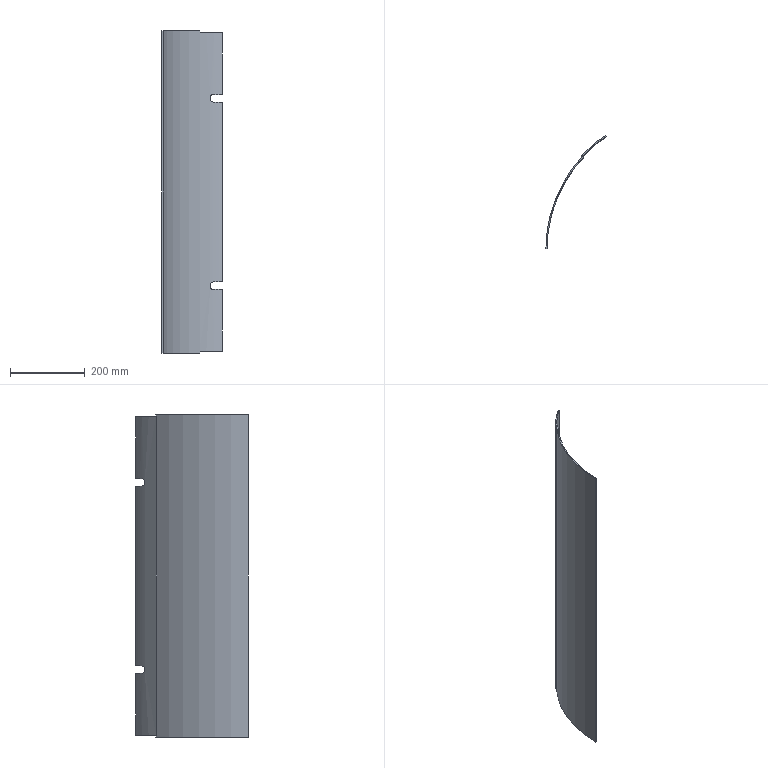Part | NX | features BREP 1 | 1 solid | 20 faces | box 160.623 x 300.85 x 860 mm | volume 907934 mm3 | plane 14 | cylinder 6 | commonest cylinder face diameters 20 x2 726 x2 720 x1 732 x1
STEP:
#1=CARTESIAN_POINT('',(-226.352,283.784,-260.));
#2=VERTEX_POINT('',#1);
#3=CARTESIAN_POINT('',(-226.352,283.784,-240.));
#4=VERTEX_POINT('',#3);
#5=CARTESIAN_POINT('',(-226.352,283.784,-260.));
#6=CARTESIAN_POINT('',(-228.418,282.137,-260.));
#7=CARTESIAN_POINT('',(-232.425,278.852,-257.834));
#8=CARTESIAN_POINT('',(-234.913,276.736,-250.009));
#9=CARTESIAN_POINT('',(-232.432,278.847,-242.169));
#10=CARTESIAN_POINT('',(-228.418,282.137,-240.));
#11=CARTESIAN_POINT('',(-226.352,283.784,-240.));
#12=B_SPLINE_CURVE_WITH_KNOTS('',3,(#5,#6,#7,#8,#9,#10,#11),.UNSPECIFIED.,.F.,.F.,(4,1,1,1,4),(0.,0.007816,0.01563,0.02345,0.03126),.UNSPECIFIED.);
#13=EDGE_CURVE('',#2,#4,#12,.T.);
#14=ORIENTED_EDGE('',*,*,#13,.T.);
#15=CARTESIAN_POINT('',(-202.365,301.36,-240.));
#16=VERTEX_POINT('',#15);
#17=CARTESIAN_POINT('',(0.,0.,-240.));
#18=DIRECTION('',(0.,0.,-1.));
#19=DIRECTION('',(-1.,0.,0.));
#20=AXIS2_PLACEMENT_3D('',#17,#18,#19);
#21=CIRCLE('',#20,363.);
#22=EDGE_CURVE('',#4,#16,#21,.T.);
#23=ORIENTED_EDGE('',*,*,#22,.T.);
#24=CARTESIAN_POINT('',(-202.365,301.36,240.));
#25=VERTEX_POINT('',#24);
#26=CARTESIAN_POINT('',(-202.365,301.36,430.));
#27=DIRECTION('',(0.,0.,-1.));
#28=VECTOR('',#27,1000.);
#29=LINE('',#26,#28);
#30=EDGE_CURVE('',#25,#16,#29,.T.);
#31=ORIENTED_EDGE('',*,*,#30,.F.);
#32=CARTESIAN_POINT('',(-226.352,283.784,240.));
#33=VERTEX_POINT('',#32);
#34=CARTESIAN_POINT('',(0.,0.,240.));
#35=DIRECTION('',(0.,0.,1.));
#36=DIRECTION('',(1.,0.,0.));
#37=AXIS2_PLACEMENT_3D('',#34,#35,#36);
#38=CIRCLE('',#37,363.);
#39=EDGE_CURVE('',#25,#33,#38,.T.);
#40=ORIENTED_EDGE('',*,*,#39,.T.);
#41=CARTESIAN_POINT('',(-226.352,283.784,260.));
#42=VERTEX_POINT('',#41);
#43=CARTESIAN_POINT('',(-226.352,283.784,240.));
#44=CARTESIAN_POINT('',(-228.418,282.137,240.));
#45=CARTESIAN_POINT('',(-232.425,278.852,242.166));
#46=CARTESIAN_POINT('',(-234.913,276.736,249.991));
#47=CARTESIAN_POINT('',(-232.432,278.847,257.831));
#48=CARTESIAN_POINT('',(-228.418,282.137,260.));
#49=CARTESIAN_POINT('',(-226.352,283.784,260.));
#50=B_SPLINE_CURVE_WITH_KNOTS('',3,(#43,#44,#45,#46,#47,#48,#49),.UNSPECIFIED.,.F.,.F.,(4,1,1,1,4),(0.,0.007816,0.01563,0.02345,0.03126),.UNSPECIFIED.);
#51=EDGE_CURVE('',#33,#42,#50,.T.);
#52=ORIENTED_EDGE('',*,*,#51,.T.);
#53=CARTESIAN_POINT('',(-202.365,301.36,260.));
#54=VERTEX_POINT('',#53);
#55=CARTESIAN_POINT('',(0.,0.,260.));
#56=DIRECTION('',(0.,0.,-1.));
#57=DIRECTION('',(-1.,0.,0.));
#58=AXIS2_PLACEMENT_3D('',#55,#56,#57);
#59=CIRCLE('',#58,363.);
#60=EDGE_CURVE('',#42,#54,#59,.T.);
#61=ORIENTED_EDGE('',*,*,#60,.T.);
#62=CARTESIAN_POINT('',(-202.365,301.36,425.));
#63=VERTEX_POINT('',#62);
#64=CARTESIAN_POINT('',(-202.365,301.36,430.));
#65=DIRECTION('',(0.,0.,-1.));
#66=VECTOR('',#65,1000.);
#67=LINE('',#64,#66);
#68=EDGE_CURVE('',#63,#54,#67,.T.);
#69=ORIENTED_EDGE('',*,*,#68,.F.);
#70=CARTESIAN_POINT('',(-263.653,249.511,425.));
#71=VERTEX_POINT('',#70);
#72=CARTESIAN_POINT('',(0.,0.,425.));
#73=DIRECTION('',(0.,0.,-1.));
#74=DIRECTION('',(1.,0.,0.));
#75=AXIS2_PLACEMENT_3D('',#72,#73,#74);
#76=CIRCLE('',#75,363.);
#77=EDGE_CURVE('',#71,#63,#76,.T.);
#78=ORIENTED_EDGE('',*,*,#77,.F.);
#79=CARTESIAN_POINT('',(-263.653,249.511,-425.));
#80=VERTEX_POINT('',#79);
#81=CARTESIAN_POINT('',(-263.653,249.511,430.));
#82=DIRECTION('',(0.,0.,-1.));
#83=VECTOR('',#82,1000.);
#84=LINE('',#81,#83);
#85=EDGE_CURVE('',#71,#80,#84,.T.);
#86=ORIENTED_EDGE('',*,*,#85,.T.);
#87=CARTESIAN_POINT('',(-202.365,301.36,-425.));
#88=VERTEX_POINT('',#87);
#89=CARTESIAN_POINT('',(0.,0.,-425.));
#90=DIRECTION('',(0.,0.,-1.));
#91=DIRECTION('',(1.,0.,0.));
#92=AXIS2_PLACEMENT_3D('',#89,#90,#91);
#93=CIRCLE('',#92,363.);
#94=EDGE_CURVE('',#80,#88,#93,.T.);
#95=ORIENTED_EDGE('',*,*,#94,.T.);
#96=CARTESIAN_POINT('',(-202.365,301.36,-260.));
#97=VERTEX_POINT('',#96);
#98=CARTESIAN_POINT('',(-202.365,301.36,430.));
#99=DIRECTION('',(0.,0.,-1.));
#100=VECTOR('',#99,1000.);
#101=LINE('',#98,#100);
#102=EDGE_CURVE('',#97,#88,#101,.T.);
#103=ORIENTED_EDGE('',*,*,#102,.F.);
#104=CARTESIAN_POINT('',(0.,0.,-260.));
#105=DIRECTION('',(0.,0.,1.));
#106=DIRECTION('',(1.,0.,0.));
#107=AXIS2_PLACEMENT_3D('',#104,#105,#106);
#108=CIRCLE('',#107,363.);
#109=EDGE_CURVE('',#97,#2,#108,.T.);
#110=ORIENTED_EDGE('',*,*,#109,.T.);
#111=EDGE_LOOP('',(#14,#23,#31,#40,#52,#61,#69,#78,#86,#95,#103,#110));
#112=FACE_BOUND('',#111,.T.);
#113=CARTESIAN_POINT('',(0.,0.,430.));
#114=DIRECTION('',(0.,0.,-1.));
#115=DIRECTION('',(1.,0.,0.));
#116=AXIS2_PLACEMENT_3D('',#113,#114,#115);
#117=CYLINDRICAL_SURFACE('',#116,363.);
#118=ADVANCED_FACE('',(#112),#117,.F.);
#119=ORIENTED_EDGE('',*,*,#30,.T.);
#120=CARTESIAN_POINT('',(-204.037,303.85,-240.));
#121=VERTEX_POINT('',#120);
#122=CARTESIAN_POINT('',(-204.037,303.85,-240.));
#123=DIRECTION('',(-0.5575,0.8302,0.));
#124=VECTOR('',#123,1000.);
#125=LINE('',#122,#124);
#126=EDGE_CURVE('',#16,#121,#125,.T.);
#127=ORIENTED_EDGE('',*,*,#126,.T.);
#128=CARTESIAN_POINT('',(-204.037,303.85,240.));
#129=VERTEX_POINT('',#128);
#130=CARTESIAN_POINT('',(-204.037,303.85,430.));
#131=DIRECTION('',(0.,0.,-1.));
#132=VECTOR('',#131,1000.);
#133=LINE('',#130,#132);
#134=EDGE_CURVE('',#129,#121,#133,.T.);
#135=ORIENTED_EDGE('',*,*,#134,.F.);
#136=CARTESIAN_POINT('',(-204.037,303.85,240.));
#137=DIRECTION('',(0.5575,-0.8302,0.));
#138=VECTOR('',#137,1000.);
#139=LINE('',#136,#138);
#140=EDGE_CURVE('',#129,#25,#139,.T.);
#141=ORIENTED_EDGE('',*,*,#140,.T.);
#142=EDGE_LOOP('',(#119,#127,#135,#141));
#143=FACE_BOUND('',#142,.T.);
#144=CARTESIAN_POINT('',(-204.037,303.85,430.));
#145=DIRECTION('',(0.8302,0.5575,0.));
#146=DIRECTION('',(0.5575,-0.8302,0.));
#147=AXIS2_PLACEMENT_3D('',#144,#145,#146);
#148=PLANE('',#147);
#149=ADVANCED_FACE('',(#143),#148,.T.);
#150=CARTESIAN_POINT('',(-204.037,303.85,-260.));
#151=VERTEX_POINT('',#150);
#152=CARTESIAN_POINT('',(-204.037,303.85,-425.));
#153=VERTEX_POINT('',#152);
#154=CARTESIAN_POINT('',(-204.037,303.85,430.));
#155=DIRECTION('',(0.,0.,-1.));
#156=VECTOR('',#155,1000.);
#157=LINE('',#154,#156);
#158=EDGE_CURVE('',#151,#153,#157,.T.);
#159=ORIENTED_EDGE('',*,*,#158,.F.);
#160=CARTESIAN_POINT('',(-204.037,303.85,-260.));
#161=DIRECTION('',(0.5575,-0.8302,0.));
#162=VECTOR('',#161,1000.);
#163=LINE('',#160,#162);
#164=EDGE_CURVE('',#151,#97,#163,.T.);
#165=ORIENTED_EDGE('',*,*,#164,.T.);
#166=ORIENTED_EDGE('',*,*,#102,.T.);
#167=CARTESIAN_POINT('',(-204.037,303.85,-425.));
#168=DIRECTION('',(-0.5575,0.8302,0.));
#169=VECTOR('',#168,1000.);
#170=LINE('',#167,#169);
#171=EDGE_CURVE('',#88,#153,#170,.T.);
#172=ORIENTED_EDGE('',*,*,#171,.T.);
#173=EDGE_LOOP('',(#159,#165,#166,#172));
#174=FACE_BOUND('',#173,.T.);
#175=CARTESIAN_POINT('',(-204.037,303.85,430.));
#176=DIRECTION('',(0.8302,0.5575,0.));
#177=DIRECTION('',(0.5575,-0.8302,0.));
#178=AXIS2_PLACEMENT_3D('',#175,#176,#177);
#179=PLANE('',#178);
#180=ADVANCED_FACE('',(#174),#179,.T.);
#181=CARTESIAN_POINT('',(-228.301,286.068,-240.));
#182=VERTEX_POINT('',#181);
#183=CARTESIAN_POINT('',(0.,0.,-240.));
#184=DIRECTION('',(0.,0.,-1.));
#185=DIRECTION('',(-1.,0.,0.));
#186=AXIS2_PLACEMENT_3D('',#183,#184,#185);
#187=CIRCLE('',#186,366.);
#188=EDGE_CURVE('',#182,#121,#187,.T.);
#189=ORIENTED_EDGE('',*,*,#188,.F.);
#190=CARTESIAN_POINT('',(-228.301,286.068,-260.));
#191=VERTEX_POINT('',#190);
#192=CARTESIAN_POINT('',(-228.301,286.068,-260.));
#193=CARTESIAN_POINT('',(-230.366,284.42,-260.));
#194=CARTESIAN_POINT('',(-234.373,281.135,-257.834));
#195=CARTESIAN_POINT('',(-236.86,279.018,-250.009));
#196=CARTESIAN_POINT('',(-234.379,281.129,-242.169));
#197=CARTESIAN_POINT('',(-230.366,284.42,-240.));
#198=CARTESIAN_POINT('',(-228.301,286.068,-240.));
#199=B_SPLINE_CURVE_WITH_KNOTS('',3,(#192,#193,#194,#195,#196,#197,#198),.UNSPECIFIED.,.F.,.F.,(4,1,1,1,4),(0.,0.007816,0.01563,0.02345,0.03126),.UNSPECIFIED.);
#200=EDGE_CURVE('',#191,#182,#199,.T.);
#201=ORIENTED_EDGE('',*,*,#200,.F.);
#202=CARTESIAN_POINT('',(0.,0.,-260.));
#203=DIRECTION('',(0.,0.,1.));
#204=DIRECTION('',(1.,0.,0.));
#205=AXIS2_PLACEMENT_3D('',#202,#203,#204);
#206=CIRCLE('',#205,366.);
#207=EDGE_CURVE('',#151,#191,#206,.T.);
#208=ORIENTED_EDGE('',*,*,#207,.F.);
#209=ORIENTED_EDGE('',*,*,#158,.T.);
#210=CARTESIAN_POINT('',(-267.83,249.445,-425.));
#211=VERTEX_POINT('',#210);
#212=CARTESIAN_POINT('',(0.,0.,-425.));
#213=DIRECTION('',(0.,0.,1.));
#214=DIRECTION('',(1.,0.,0.));
#215=AXIS2_PLACEMENT_3D('',#212,#213,#214);
#216=CIRCLE('',#215,366.);
#217=EDGE_CURVE('',#153,#211,#216,.T.);
#218=ORIENTED_EDGE('',*,*,#217,.T.);
#219=CARTESIAN_POINT('',(-267.83,249.445,425.));
#220=VERTEX_POINT('',#219);
#221=CARTESIAN_POINT('',(-267.83,249.445,430.));
#222=DIRECTION('',(0.,0.,-1.));
#223=VECTOR('',#222,1000.);
#224=LINE('',#221,#223);
#225=EDGE_CURVE('',#220,#211,#224,.T.);
#226=ORIENTED_EDGE('',*,*,#225,.F.);
#227=CARTESIAN_POINT('',(-204.037,303.85,425.));
#228=VERTEX_POINT('',#227);
#229=CARTESIAN_POINT('',(0.,0.,425.));
#230=DIRECTION('',(0.,0.,1.));
#231=DIRECTION('',(1.,0.,0.));
#232=AXIS2_PLACEMENT_3D('',#229,#230,#231);
#233=CIRCLE('',#232,366.);
#234=EDGE_CURVE('',#228,#220,#233,.T.);
#235=ORIENTED_EDGE('',*,*,#234,.F.);
#236=CARTESIAN_POINT('',(-204.037,303.85,260.));
#237=VERTEX_POINT('',#236);
#238=CARTESIAN_POINT('',(-204.037,303.85,430.));
#239=DIRECTION('',(0.,0.,-1.));
#240=VECTOR('',#239,1000.);
#241=LINE('',#238,#240);
#242=EDGE_CURVE('',#228,#237,#241,.T.);
#243=ORIENTED_EDGE('',*,*,#242,.T.);
#244=CARTESIAN_POINT('',(-228.301,286.068,260.));
#245=VERTEX_POINT('',#244);
#246=CARTESIAN_POINT('',(0.,0.,260.));
#247=DIRECTION('',(0.,0.,-1.));
#248=DIRECTION('',(-1.,0.,0.));
#249=AXIS2_PLACEMENT_3D('',#246,#247,#248);
#250=CIRCLE('',#249,366.);
#251=EDGE_CURVE('',#245,#237,#250,.T.);
#252=ORIENTED_EDGE('',*,*,#251,.F.);
#253=CARTESIAN_POINT('',(-228.301,286.068,240.));
#254=VERTEX_POINT('',#253);
#255=CARTESIAN_POINT('',(-228.301,286.068,240.));
#256=CARTESIAN_POINT('',(-230.366,284.42,240.));
#257=CARTESIAN_POINT('',(-234.373,281.135,242.166));
#258=CARTESIAN_POINT('',(-236.86,279.018,249.991));
#259=CARTESIAN_POINT('',(-234.379,281.129,257.831));
#260=CARTESIAN_POINT('',(-230.366,284.42,260.));
#261=CARTESIAN_POINT('',(-228.301,286.068,260.));
#262=B_SPLINE_CURVE_WITH_KNOTS('',3,(#255,#256,#257,#258,#259,#260,#261),.UNSPECIFIED.,.F.,.F.,(4,1,1,1,4),(0.,0.007816,0.01563,0.02345,0.03126),.UNSPECIFIED.);
#263=EDGE_CURVE('',#254,#245,#262,.T.);
#264=ORIENTED_EDGE('',*,*,#263,.F.);
#265=CARTESIAN_POINT('',(0.,0.,240.));
#266=DIRECTION('',(0.,0.,1.));
#267=DIRECTION('',(1.,0.,0.));
#268=AXIS2_PLACEMENT_3D('',#265,#266,#267);
#269=CIRCLE('',#268,366.);
#270=EDGE_CURVE('',#129,#254,#269,.T.);
#271=ORIENTED_EDGE('',*,*,#270,.F.);
#272=ORIENTED_EDGE('',*,*,#134,.T.);
#273=EDGE_LOOP('',(#189,#201,#208,#209,#218,#226,#235,#243,#252,#264,#271,#272));
#274=FACE_BOUND('',#273,.T.);
#275=CARTESIAN_POINT('',(0.,0.,430.));
#276=DIRECTION('',(0.,0.,-1.));
#277=DIRECTION('',(1.,0.,0.));
#278=AXIS2_PLACEMENT_3D('',#275,#276,#277);
#279=CYLINDRICAL_SURFACE('',#278,366.);
#280=ADVANCED_FACE('',(#274),#279,.T.);
#281=ORIENTED_EDGE('',*,*,#68,.T.);
#282=CARTESIAN_POINT('',(-204.037,303.85,260.));
#283=DIRECTION('',(-0.5575,0.8302,0.));
#284=VECTOR('',#283,1000.);
#285=LINE('',#282,#284);
#286=EDGE_CURVE('',#54,#237,#285,.T.);
#287=ORIENTED_EDGE('',*,*,#286,.T.);
#288=ORIENTED_EDGE('',*,*,#242,.F.);
#289=CARTESIAN_POINT('',(-204.037,303.85,425.));
#290=DIRECTION('',(-0.5575,0.8302,0.));
#291=VECTOR('',#290,1000.);
#292=LINE('',#289,#291);
#293=EDGE_CURVE('',#63,#228,#292,.T.);
#294=ORIENTED_EDGE('',*,*,#293,.F.);
#295=EDGE_LOOP('',(#281,#287,#288,#294));
#296=FACE_BOUND('',#295,.T.);
#297=CARTESIAN_POINT('',(-204.037,303.85,430.));
#298=DIRECTION('',(0.8302,0.5575,0.));
#299=DIRECTION('',(0.5575,-0.8302,0.));
#300=AXIS2_PLACEMENT_3D('',#297,#298,#299);
#301=PLANE('',#300);
#302=ADVANCED_FACE('',(#296),#301,.T.);
#303=CARTESIAN_POINT('',(-265.707,247.323,-425.));
#304=VERTEX_POINT('',#303);
#305=CARTESIAN_POINT('',(-267.83,249.445,-425.));
#306=DIRECTION('',(0.7071,-0.7071,0.));
#307=VECTOR('',#306,1000.);
#308=LINE('',#305,#307);
#309=EDGE_CURVE('',#211,#304,#308,.T.);
#310=ORIENTED_EDGE('',*,*,#309,.T.);
#311=CARTESIAN_POINT('',(-265.707,247.323,425.));
#312=VERTEX_POINT('',#311);
#313=CARTESIAN_POINT('',(-265.707,247.323,430.));
#314=DIRECTION('',(0.,0.,-1.));
#315=VECTOR('',#314,1000.);
#316=LINE('',#313,#315);
#317=EDGE_CURVE('',#312,#304,#316,.T.);
#318=ORIENTED_EDGE('',*,*,#317,.F.);
#319=CARTESIAN_POINT('',(-267.83,249.445,425.));
#320=DIRECTION('',(0.7071,-0.7071,0.));
#321=VECTOR('',#320,1000.);
#322=LINE('',#319,#321);
#323=EDGE_CURVE('',#220,#312,#322,.T.);
#324=ORIENTED_EDGE('',*,*,#323,.F.);
#325=ORIENTED_EDGE('',*,*,#225,.T.);
#326=EDGE_LOOP('',(#310,#318,#324,#325));
#327=FACE_BOUND('',#326,.T.);
#328=CARTESIAN_POINT('',(-263.653,245.268,430.));
#329=DIRECTION('',(0.7071,0.7071,0.));
#330=DIRECTION('',(0.7071,-0.7071,0.));
#331=AXIS2_PLACEMENT_3D('',#328,#329,#330);
#332=PLANE('',#331);
#333=ADVANCED_FACE('',(#327),#332,.F.);
#334=CARTESIAN_POINT('',(-263.653,249.511,430.));
#335=VERTEX_POINT('',#334);
#336=CARTESIAN_POINT('',(-261.531,247.389,430.));
#337=VERTEX_POINT('',#336);
#338=CARTESIAN_POINT('',(-261.531,247.389,430.));
#339=DIRECTION('',(0.7071,-0.7071,0.));
#340=VECTOR('',#339,1000.);
#341=LINE('',#338,#340);
#342=EDGE_CURVE('',#335,#337,#341,.T.);
#343=ORIENTED_EDGE('',*,*,#342,.F.);
#344=CARTESIAN_POINT('',(-362.987,3.025,430.));
#345=VERTEX_POINT('',#344);
#346=CARTESIAN_POINT('',(0.,0.,430.));
#347=DIRECTION('',(0.,0.,1.));
#348=DIRECTION('',(1.,0.,0.));
#349=AXIS2_PLACEMENT_3D('',#346,#347,#348);
#350=CIRCLE('',#349,363.);
#351=EDGE_CURVE('',#335,#345,#350,.T.);
#352=ORIENTED_EDGE('',*,*,#351,.T.);
#353=CARTESIAN_POINT('',(-359.987,3.,430.));
#354=VERTEX_POINT('',#353);
#355=CARTESIAN_POINT('',(-359.987,3.,430.));
#356=DIRECTION('',(-1.,0.008333,0.));
#357=VECTOR('',#356,1000.);
#358=LINE('',#355,#357);
#359=EDGE_CURVE('',#354,#345,#358,.T.);
#360=ORIENTED_EDGE('',*,*,#359,.F.);
#361=CARTESIAN_POINT('',(0.,0.,430.));
#362=DIRECTION('',(0.,0.,1.));
#363=DIRECTION('',(1.,0.,0.));
#364=AXIS2_PLACEMENT_3D('',#361,#362,#363);
#365=CIRCLE('',#364,360.);
#366=EDGE_CURVE('',#337,#354,#365,.T.);
#367=ORIENTED_EDGE('',*,*,#366,.F.);
#368=EDGE_LOOP('',(#343,#352,#360,#367));
#369=FACE_BOUND('',#368,.T.);
#370=CARTESIAN_POINT('',(0.,0.,430.));
#371=DIRECTION('',(0.,0.,1.));
#372=DIRECTION('',(-1.,0.,0.));
#373=AXIS2_PLACEMENT_3D('',#370,#371,#372);
#374=PLANE('',#373);
#375=ADVANCED_FACE('',(#369),#374,.T.);
#376=CARTESIAN_POINT('',(-263.653,249.511,-430.));
#377=VERTEX_POINT('',#376);
#378=CARTESIAN_POINT('',(-362.987,3.025,-430.));
#379=VERTEX_POINT('',#378);
#380=CARTESIAN_POINT('',(0.,0.,-430.));
#381=DIRECTION('',(0.,0.,1.));
#382=DIRECTION('',(1.,0.,0.));
#383=AXIS2_PLACEMENT_3D('',#380,#381,#382);
#384=CIRCLE('',#383,363.);
#385=EDGE_CURVE('',#377,#379,#384,.T.);
#386=ORIENTED_EDGE('',*,*,#385,.T.);
#387=CARTESIAN_POINT('',(-362.987,3.025,430.));
#388=DIRECTION('',(0.,0.,-1.));
#389=VECTOR('',#388,1000.);
#390=LINE('',#387,#389);
#391=EDGE_CURVE('',#345,#379,#390,.T.);
#392=ORIENTED_EDGE('',*,*,#391,.F.);
#393=ORIENTED_EDGE('',*,*,#351,.F.);
#394=CARTESIAN_POINT('',(-263.653,249.511,430.));
#395=DIRECTION('',(0.,0.,-1.));
#396=VECTOR('',#395,1000.);
#397=LINE('',#394,#396);
#398=EDGE_CURVE('',#335,#71,#397,.T.);
#399=ORIENTED_EDGE('',*,*,#398,.T.);
#400=CARTESIAN_POINT('',(0.,0.,425.));
#401=DIRECTION('',(0.,0.,-1.));
#402=DIRECTION('',(1.,0.,0.));
#403=AXIS2_PLACEMENT_3D('',#400,#401,#402);
#404=CIRCLE('',#403,363.);
#405=EDGE_CURVE('',#312,#71,#404,.T.);
#406=ORIENTED_EDGE('',*,*,#405,.F.);
#407=ORIENTED_EDGE('',*,*,#317,.T.);
#408=CARTESIAN_POINT('',(0.,0.,-425.));
#409=DIRECTION('',(0.,0.,-1.));
#410=DIRECTION('',(1.,0.,0.));
#411=AXIS2_PLACEMENT_3D('',#408,#409,#410);
#412=CIRCLE('',#411,363.);
#413=EDGE_CURVE('',#304,#80,#412,.T.);
#414=ORIENTED_EDGE('',*,*,#413,.T.);
#415=CARTESIAN_POINT('',(-263.653,249.511,-430.));
#416=DIRECTION('',(0.,0.,-1.));
#417=VECTOR('',#416,1000.);
#418=LINE('',#415,#417);
#419=EDGE_CURVE('',#80,#377,#418,.T.);
#420=ORIENTED_EDGE('',*,*,#419,.T.);
#421=EDGE_LOOP('',(#386,#392,#393,#399,#406,#407,#414,#420));
#422=FACE_BOUND('',#421,.T.);
#423=CARTESIAN_POINT('',(0.,0.,430.));
#424=DIRECTION('',(0.,0.,-1.));
#425=DIRECTION('',(1.,0.,0.));
#426=AXIS2_PLACEMENT_3D('',#423,#424,#425);
#427=CYLINDRICAL_SURFACE('',#426,363.);
#428=ADVANCED_FACE('',(#422),#427,.T.);
#429=CARTESIAN_POINT('',(-359.987,3.,-430.));
#430=VERTEX_POINT('',#429);
#431=CARTESIAN_POINT('',(-359.987,3.,-430.));
#432=DIRECTION('',(-1.,0.008333,0.));
#433=VECTOR('',#432,1000.);
#434=LINE('',#431,#433);
#435=EDGE_CURVE('',#430,#379,#434,.T.);
#436=ORIENTED_EDGE('',*,*,#435,.F.);
#437=CARTESIAN_POINT('',(-359.987,3.,430.));
#438=DIRECTION('',(0.,0.,-1.));
#439=VECTOR('',#438,1000.);
#440=LINE('',#437,#439);
#441=EDGE_CURVE('',#354,#430,#440,.T.);
#442=ORIENTED_EDGE('',*,*,#441,.F.);
#443=ORIENTED_EDGE('',*,*,#359,.T.);
#444=ORIENTED_EDGE('',*,*,#391,.T.);
#445=EDGE_LOOP('',(#436,#442,#443,#444));
#446=FACE_BOUND('',#445,.T.);
#447=CARTESIAN_POINT('',(-359.987,3.,430.));
#448=DIRECTION('',(-0.008333,-1.,0.));
#449=DIRECTION('',(-1.,0.008333,0.));
#450=AXIS2_PLACEMENT_3D('',#447,#448,#449);
#451=PLANE('',#450);
#452=ADVANCED_FACE('',(#446),#451,.T.);
#453=CARTESIAN_POINT('',(-261.531,247.389,-430.));
#454=VERTEX_POINT('',#453);
#455=CARTESIAN_POINT('',(0.,0.,-430.));
#456=DIRECTION('',(0.,0.,1.));
#457=DIRECTION('',(1.,0.,0.));
#458=AXIS2_PLACEMENT_3D('',#455,#456,#457);
#459=CIRCLE('',#458,360.);
#460=EDGE_CURVE('',#454,#430,#459,.T.);
#461=ORIENTED_EDGE('',*,*,#460,.F.);
#462=CARTESIAN_POINT('',(-261.531,247.389,430.));
#463=DIRECTION('',(0.,0.,-1.));
#464=VECTOR('',#463,1000.);
#465=LINE('',#462,#464);
#466=EDGE_CURVE('',#337,#454,#465,.T.);
#467=ORIENTED_EDGE('',*,*,#466,.F.);
#468=ORIENTED_EDGE('',*,*,#366,.T.);
#469=ORIENTED_EDGE('',*,*,#441,.T.);
#470=EDGE_LOOP('',(#461,#467,#468,#469));
#471=FACE_BOUND('',#470,.T.);
#472=CARTESIAN_POINT('',(0.,0.,430.));
#473=DIRECTION('',(0.,0.,-1.));
#474=DIRECTION('',(1.,0.,0.));
#475=AXIS2_PLACEMENT_3D('',#472,#473,#474);
#476=CYLINDRICAL_SURFACE('',#475,360.);
#477=ADVANCED_FACE('',(#471),#476,.F.);
#478=CARTESIAN_POINT('',(-261.531,247.389,-430.));
#479=DIRECTION('',(0.7071,-0.7071,0.));
#480=VECTOR('',#479,1000.);
#481=LINE('',#478,#480);
#482=EDGE_CURVE('',#377,#454,#481,.T.);
#483=ORIENTED_EDGE('',*,*,#482,.F.);
#484=ORIENTED_EDGE('',*,*,#419,.F.);
#485=ORIENTED_EDGE('',*,*,#85,.F.);
#486=ORIENTED_EDGE('',*,*,#398,.F.);
#487=ORIENTED_EDGE('',*,*,#342,.T.);
#488=ORIENTED_EDGE('',*,*,#466,.T.);
#489=EDGE_LOOP('',(#483,#484,#485,#486,#487,#488));
#490=FACE_BOUND('',#489,.T.);
#491=CARTESIAN_POINT('',(-261.531,247.389,430.));
#492=DIRECTION('',(0.7071,0.7071,0.));
#493=DIRECTION('',(0.7071,-0.7071,0.));
#494=AXIS2_PLACEMENT_3D('',#491,#492,#493);
#495=PLANE('',#494);
#496=ADVANCED_FACE('',(#490),#495,.T.);
#497=ORIENTED_EDGE('',*,*,#385,.F.);
#498=ORIENTED_EDGE('',*,*,#482,.T.);
#499=ORIENTED_EDGE('',*,*,#460,.T.);
#500=ORIENTED_EDGE('',*,*,#435,.T.);
#501=EDGE_LOOP('',(#497,#498,#499,#500));
#502=FACE_BOUND('',#501,.T.);
#503=CARTESIAN_POINT('',(0.,0.,-430.));
#504=DIRECTION('',(0.,0.,1.));
#505=DIRECTION('',(-1.,0.,0.));
#506=AXIS2_PLACEMENT_3D('',#503,#504,#505);
#507=PLANE('',#506);
#508=ADVANCED_FACE('',(#502),#507,.F.);
#509=ORIENTED_EDGE('',*,*,#405,.T.);
#510=ORIENTED_EDGE('',*,*,#77,.T.);
#511=ORIENTED_EDGE('',*,*,#293,.T.);
#512=ORIENTED_EDGE('',*,*,#234,.T.);
#513=ORIENTED_EDGE('',*,*,#323,.T.);
#514=EDGE_LOOP('',(#509,#510,#511,#512,#513));
#515=FACE_BOUND('',#514,.T.);
#516=CARTESIAN_POINT('',(0.,0.,425.));
#517=DIRECTION('',(0.,0.,1.));
#518=DIRECTION('',(-1.,0.,0.));
#519=AXIS2_PLACEMENT_3D('',#516,#517,#518);
#520=PLANE('',#519);
#521=ADVANCED_FACE('',(#515),#520,.T.);
#522=ORIENTED_EDGE('',*,*,#413,.F.);
#523=ORIENTED_EDGE('',*,*,#309,.F.);
#524=ORIENTED_EDGE('',*,*,#217,.F.);
#525=ORIENTED_EDGE('',*,*,#171,.F.);
#526=ORIENTED_EDGE('',*,*,#94,.F.);
#527=EDGE_LOOP('',(#522,#523,#524,#525,#526));
#528=FACE_BOUND('',#527,.T.);
#529=CARTESIAN_POINT('',(0.,0.,-425.));
#530=DIRECTION('',(0.,0.,-1.));
#531=DIRECTION('',(-1.,0.,0.));
#532=AXIS2_PLACEMENT_3D('',#529,#530,#531);
#533=PLANE('',#532);
#534=ADVANCED_FACE('',(#528),#533,.T.);
#535=CARTESIAN_POINT('',(-293.812,362.862,240.));
#536=DIRECTION('',(0.649,-0.7608,0.));
#537=VECTOR('',#536,1000.);
#538=LINE('',#535,#537);
#539=EDGE_CURVE('',#254,#33,#538,.T.);
#540=ORIENTED_EDGE('',*,*,#539,.F.);
#541=ORIENTED_EDGE('',*,*,#263,.T.);
#542=CARTESIAN_POINT('',(-293.812,362.862,260.));
#543=DIRECTION('',(0.649,-0.7608,0.));
#544=VECTOR('',#543,1000.);
#545=LINE('',#542,#544);
#546=EDGE_CURVE('',#245,#42,#545,.T.);
#547=ORIENTED_EDGE('',*,*,#546,.T.);
#548=ORIENTED_EDGE('',*,*,#51,.F.);
#549=EDGE_LOOP('',(#540,#541,#547,#548));
#550=FACE_BOUND('',#549,.T.);
#551=CARTESIAN_POINT('',(-293.812,362.862,250.));
#552=DIRECTION('',(0.649,-0.7608,0.));
#553=DIRECTION('',(-0.7608,-0.649,0.));
#554=AXIS2_PLACEMENT_3D('',#551,#552,#553);
#555=CYLINDRICAL_SURFACE('',#554,10.);
#556=ADVANCED_FACE('',(#550),#555,.F.);
#557=ORIENTED_EDGE('',*,*,#546,.F.);
#558=ORIENTED_EDGE('',*,*,#251,.T.);
#559=ORIENTED_EDGE('',*,*,#286,.F.);
#560=ORIENTED_EDGE('',*,*,#60,.F.);
#561=EDGE_LOOP('',(#557,#558,#559,#560));
#562=FACE_BOUND('',#561,.T.);
#563=CARTESIAN_POINT('',(-293.812,362.862,260.));
#564=DIRECTION('',(0.,0.,-1.));
#565=DIRECTION('',(1.,0.,0.));
#566=AXIS2_PLACEMENT_3D('',#563,#564,#565);
#567=PLANE('',#566);
#568=ADVANCED_FACE('',(#562),#567,.T.);
#569=ORIENTED_EDGE('',*,*,#140,.F.);
#570=ORIENTED_EDGE('',*,*,#270,.T.);
#571=ORIENTED_EDGE('',*,*,#539,.T.);
#572=ORIENTED_EDGE('',*,*,#39,.F.);
#573=EDGE_LOOP('',(#569,#570,#571,#572));
#574=FACE_BOUND('',#573,.T.);
#575=CARTESIAN_POINT('',(-263.361,388.84,240.));
#576=DIRECTION('',(0.,0.,1.));
#577=DIRECTION('',(-1.,0.,0.));
#578=AXIS2_PLACEMENT_3D('',#575,#576,#577);
#579=PLANE('',#578);
#580=ADVANCED_FACE('',(#574),#579,.T.);
#581=CARTESIAN_POINT('',(-293.812,362.862,-260.));
#582=DIRECTION('',(0.649,-0.7608,0.));
#583=VECTOR('',#582,1000.);
#584=LINE('',#581,#583);
#585=EDGE_CURVE('',#191,#2,#584,.T.);
#586=ORIENTED_EDGE('',*,*,#585,.F.);
#587=ORIENTED_EDGE('',*,*,#200,.T.);
#588=CARTESIAN_POINT('',(-293.812,362.862,-240.));
#589=DIRECTION('',(0.649,-0.7608,0.));
#590=VECTOR('',#589,1000.);
#591=LINE('',#588,#590);
#592=EDGE_CURVE('',#182,#4,#591,.T.);
#593=ORIENTED_EDGE('',*,*,#592,.T.);
#594=ORIENTED_EDGE('',*,*,#13,.F.);
#595=EDGE_LOOP('',(#586,#587,#593,#594));
#596=FACE_BOUND('',#595,.T.);
#597=CARTESIAN_POINT('',(-293.812,362.862,-250.));
#598=DIRECTION('',(0.649,-0.7608,0.));
#599=DIRECTION('',(-0.7608,-0.649,0.));
#600=AXIS2_PLACEMENT_3D('',#597,#598,#599);
#601=CYLINDRICAL_SURFACE('',#600,10.);
#602=ADVANCED_FACE('',(#596),#601,.F.);
#603=ORIENTED_EDGE('',*,*,#592,.F.);
#604=ORIENTED_EDGE('',*,*,#188,.T.);
#605=ORIENTED_EDGE('',*,*,#126,.F.);
#606=ORIENTED_EDGE('',*,*,#22,.F.);
#607=EDGE_LOOP('',(#603,#604,#605,#606));
#608=FACE_BOUND('',#607,.T.);
#609=CARTESIAN_POINT('',(-263.361,388.84,-240.));
#610=DIRECTION('',(0.,0.,-1.));
#611=DIRECTION('',(1.,0.,0.));
#612=AXIS2_PLACEMENT_3D('',#609,#610,#611);
#613=PLANE('',#612);
#614=ADVANCED_FACE('',(#608),#613,.T.);
#615=ORIENTED_EDGE('',*,*,#164,.F.);
#616=ORIENTED_EDGE('',*,*,#207,.T.);
#617=ORIENTED_EDGE('',*,*,#585,.T.);
#618=ORIENTED_EDGE('',*,*,#109,.F.);
#619=EDGE_LOOP('',(#615,#616,#617,#618));
#620=FACE_BOUND('',#619,.T.);
#621=CARTESIAN_POINT('',(-293.812,362.862,-260.));
#622=DIRECTION('',(0.,0.,1.));
#623=DIRECTION('',(-1.,0.,0.));
#624=AXIS2_PLACEMENT_3D('',#621,#622,#623);
#625=PLANE('',#624);
#626=ADVANCED_FACE('',(#620),#625,.T.);
#627=CLOSED_SHELL('',(#118,#149,#180,#280,#302,#333,#375,#428,#452,#477,#496,#508,#521,#534,#556,#568,#580,#602,#614,#626));
#628=MANIFOLD_SOLID_BREP('',#627);
#629=(LENGTH_UNIT()NAMED_UNIT(*)SI_UNIT(.MILLI.,.METRE.));
#630=UNCERTAINTY_MEASURE_WITH_UNIT(LENGTH_MEASURE(0.0508),#629,'','');
#631=(NAMED_UNIT(*)PLANE_ANGLE_UNIT()SI_UNIT($,.RADIAN.));
#632=(NAMED_UNIT(*)SI_UNIT($,.STERADIAN.)SOLID_ANGLE_UNIT());
#633=(GEOMETRIC_REPRESENTATION_CONTEXT(3)GLOBAL_UNCERTAINTY_ASSIGNED_CONTEXT((#630))GLOBAL_UNIT_ASSIGNED_CONTEXT((#629,#631,#632))REPRESENTATION_CONTEXT('',''));
#634=ADVANCED_BREP_SHAPE_REPRESENTATION('',(#628),#633);